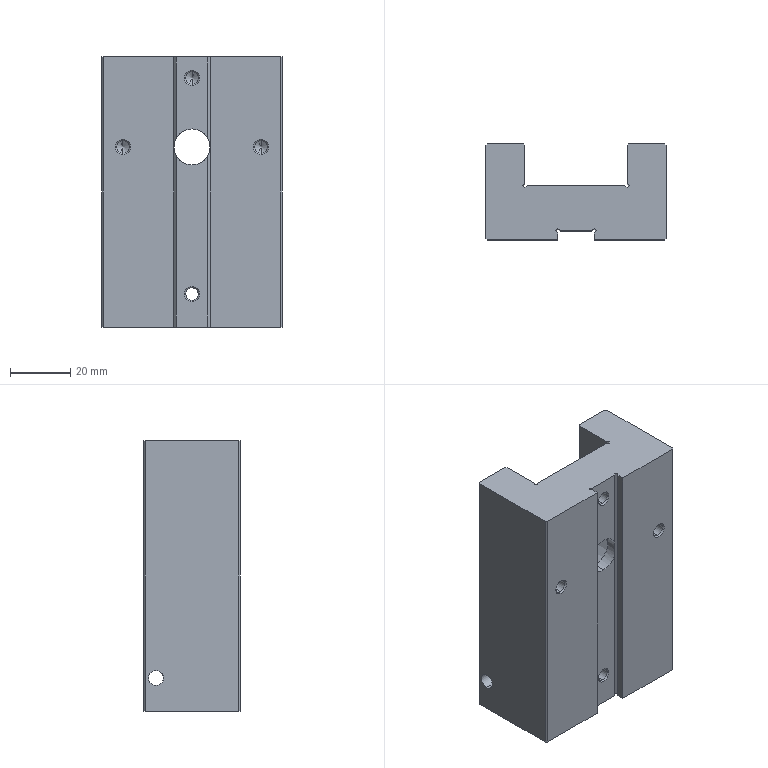Part | SolidWorks | features 3DProfileFeature 4, HoleWzd 4, ICE 3, Extrusion 1 | 1 solid | 116 faces | box 60 x 32 x 90 mm | volume 115385 mm3 | plane 44 | cone 40 | cylinder 32 | commonest cylinder face diameters 6.8 x12 4.2 x8 5 x4 36 x4 12 x2 23 x2